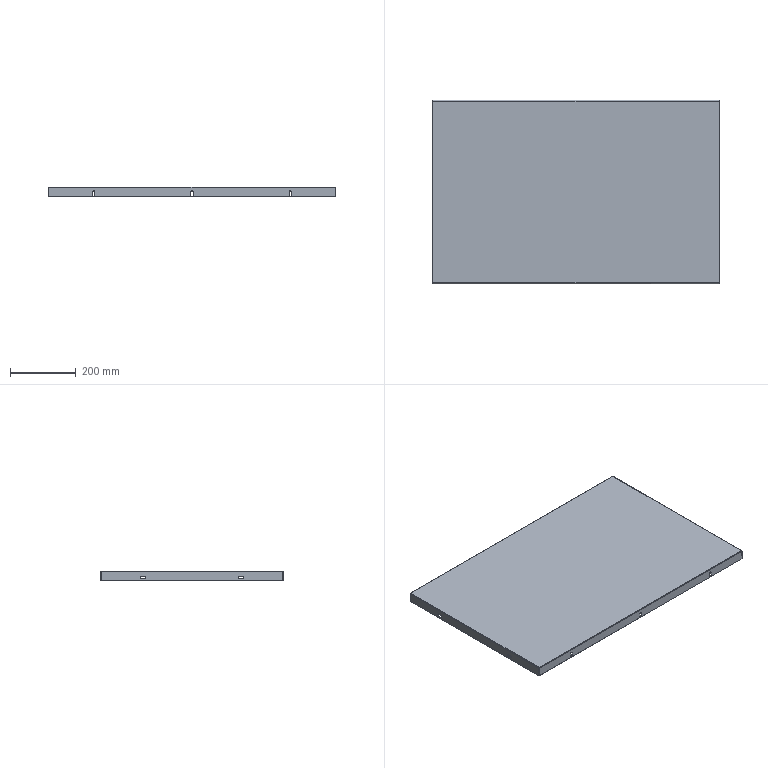Part | SolidWorks | features BaseBody 1 | 1 solid | 84 faces | box 878 x 560 x 30 mm | volume 855322 mm3 | plane 42 | cylinder 34 | spline 8 | commonest cylinder face diameters 7 x26 1.473 x4 4.473 x4